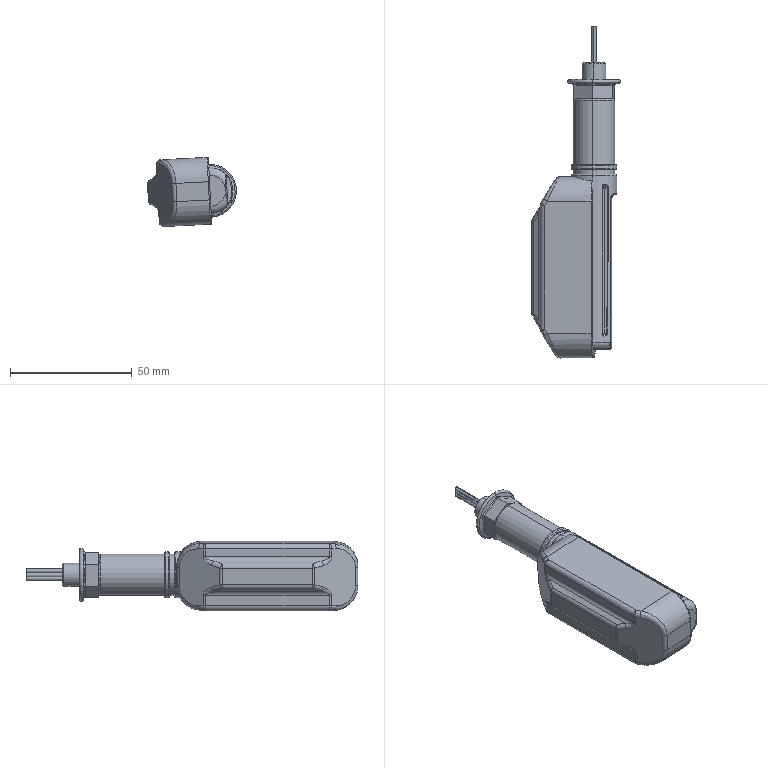Part | SolidWorks | features BaseBody 1 | 1 solid | 191 faces | box 36.572 x 136.5 x 28.449 mm | volume 38986 mm3 | cylinder 72 | plane 58 | spline 28 | torus 21 | sphere 8 | cone 4 | commonest cylinder face diameters 4 x23 1 x7 1.55 x6 12 x6 1.5 x5 18.8 x5